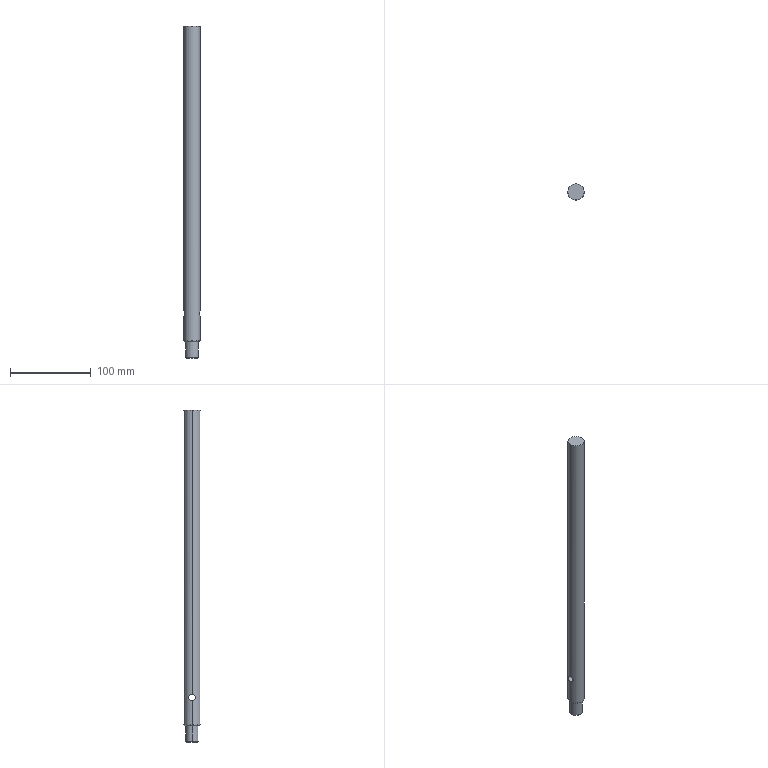Part | SolidWorks | features ICE 4, Chamfer 1, Revolution 1 | 1 solid | 13 faces | box 20 x 20 x 410 mm | volume 125504 mm3 | cylinder 6 | cone 4 | plane 3 | commonest cylinder face diameters 8 x2 16 x2 20 x2
STEP:
#1=CARTESIAN_POINT('',(-7.,0.,-190.));
#2=VERTEX_POINT('',#1);
#3=CARTESIAN_POINT('',(7.,0.,-190.));
#4=VERTEX_POINT('',#3);
#5=CARTESIAN_POINT('',(0.,0.,-190.));
#6=DIRECTION('',(0.,0.,-1.));
#7=DIRECTION('',(-1.,0.,0.));
#8=AXIS2_PLACEMENT_3D('',#5,#6,#7);
#9=CIRCLE('',#8,7.);
#10=EDGE_CURVE('',#2,#4,#9,.T.);
#11=ORIENTED_EDGE('',*,*,#10,.F.);
#12=CARTESIAN_POINT('',(-8.,0.,-189.));
#13=VERTEX_POINT('',#12);
#14=CARTESIAN_POINT('',(-7.,0.,-190.));
#15=DIRECTION('',(-0.7071,0.,0.7071));
#16=VECTOR('',#15,1000.);
#17=LINE('',#14,#16);
#18=EDGE_CURVE('',#2,#13,#17,.T.);
#19=ORIENTED_EDGE('',*,*,#18,.T.);
#20=CARTESIAN_POINT('',(8.,0.,-189.));
#21=VERTEX_POINT('',#20);
#22=CARTESIAN_POINT('',(0.,0.,-189.));
#23=DIRECTION('',(0.,0.,1.));
#24=DIRECTION('',(-1.,0.,0.));
#25=AXIS2_PLACEMENT_3D('',#22,#23,#24);
#26=CIRCLE('',#25,8.);
#27=EDGE_CURVE('',#21,#13,#26,.T.);
#28=ORIENTED_EDGE('',*,*,#27,.F.);
#29=CARTESIAN_POINT('',(7.,0.,-190.));
#30=DIRECTION('',(0.7071,0.,0.7071));
#31=VECTOR('',#30,1000.);
#32=LINE('',#29,#31);
#33=EDGE_CURVE('',#4,#21,#32,.T.);
#34=ORIENTED_EDGE('',*,*,#33,.F.);
#35=EDGE_LOOP('',(#11,#19,#28,#34));
#36=FACE_OUTER_BOUND('',#35,.T.);
#37=CARTESIAN_POINT('',(0.,0.,-190.));
#38=DIRECTION('',(0.,0.,1.));
#39=DIRECTION('',(1.,0.,0.));
#40=AXIS2_PLACEMENT_3D('',#37,#38,#39);
#41=CONICAL_SURFACE('',#40,7.,0.7854);
#42=ADVANCED_FACE('',(#36),#41,.T.);
#43=CARTESIAN_POINT('',(-9.,0.,-170.));
#44=VERTEX_POINT('',#43);
#45=CARTESIAN_POINT('',(9.,0.,-170.));
#46=VERTEX_POINT('',#45);
#47=CARTESIAN_POINT('',(0.,0.,-170.));
#48=DIRECTION('',(0.,0.,-1.));
#49=DIRECTION('',(-1.,0.,0.));
#50=AXIS2_PLACEMENT_3D('',#47,#48,#49);
#51=CIRCLE('',#50,9.);
#52=EDGE_CURVE('',#44,#46,#51,.T.);
#53=ORIENTED_EDGE('',*,*,#52,.F.);
#54=CARTESIAN_POINT('',(-10.,0.,-169.));
#55=VERTEX_POINT('',#54);
#56=CARTESIAN_POINT('',(-9.,0.,-170.));
#57=DIRECTION('',(-0.7071,0.,0.7071));
#58=VECTOR('',#57,1000.);
#59=LINE('',#56,#58);
#60=EDGE_CURVE('',#44,#55,#59,.T.);
#61=ORIENTED_EDGE('',*,*,#60,.T.);
#62=CARTESIAN_POINT('',(10.,0.,-169.));
#63=VERTEX_POINT('',#62);
#64=CARTESIAN_POINT('',(0.,0.,-169.));
#65=DIRECTION('',(0.,0.,1.));
#66=DIRECTION('',(-1.,0.,0.));
#67=AXIS2_PLACEMENT_3D('',#64,#65,#66);
#68=CIRCLE('',#67,10.);
#69=EDGE_CURVE('',#63,#55,#68,.T.);
#70=ORIENTED_EDGE('',*,*,#69,.F.);
#71=CARTESIAN_POINT('',(9.,0.,-170.));
#72=DIRECTION('',(0.7071,0.,0.7071));
#73=VECTOR('',#72,1000.);
#74=LINE('',#71,#73);
#75=EDGE_CURVE('',#46,#63,#74,.T.);
#76=ORIENTED_EDGE('',*,*,#75,.F.);
#77=EDGE_LOOP('',(#53,#61,#70,#76));
#78=FACE_OUTER_BOUND('',#77,.T.);
#79=CARTESIAN_POINT('',(0.,0.,-170.));
#80=DIRECTION('',(0.,0.,1.));
#81=DIRECTION('',(1.,0.,0.));
#82=AXIS2_PLACEMENT_3D('',#79,#80,#81);
#83=CONICAL_SURFACE('',#82,9.,0.7854);
#84=ADVANCED_FACE('',(#78),#83,.T.);
#85=ORIENTED_EDGE('',*,*,#27,.T.);
#86=CARTESIAN_POINT('',(-8.,0.,-170.));
#87=VERTEX_POINT('',#86);
#88=CARTESIAN_POINT('',(-8.,0.,-190.));
#89=DIRECTION('',(0.,0.,1.));
#90=VECTOR('',#89,1000.);
#91=LINE('',#88,#90);
#92=EDGE_CURVE('',#13,#87,#91,.T.);
#93=ORIENTED_EDGE('',*,*,#92,.T.);
#94=CARTESIAN_POINT('',(8.,0.,-170.));
#95=VERTEX_POINT('',#94);
#96=CARTESIAN_POINT('',(0.,0.,-170.));
#97=DIRECTION('',(0.,0.,-1.));
#98=DIRECTION('',(-1.,0.,0.));
#99=AXIS2_PLACEMENT_3D('',#96,#97,#98);
#100=CIRCLE('',#99,8.);
#101=EDGE_CURVE('',#87,#95,#100,.T.);
#102=ORIENTED_EDGE('',*,*,#101,.T.);
#103=CARTESIAN_POINT('',(8.,0.,-190.));
#104=DIRECTION('',(0.,0.,1.));
#105=VECTOR('',#104,1000.);
#106=LINE('',#103,#105);
#107=EDGE_CURVE('',#21,#95,#106,.T.);
#108=ORIENTED_EDGE('',*,*,#107,.F.);
#109=EDGE_LOOP('',(#85,#93,#102,#108));
#110=FACE_OUTER_BOUND('',#109,.T.);
#111=CARTESIAN_POINT('',(0.,0.,-190.));
#112=DIRECTION('',(0.,0.,1.));
#113=DIRECTION('',(1.,0.,0.));
#114=AXIS2_PLACEMENT_3D('',#111,#112,#113);
#115=CYLINDRICAL_SURFACE('',#114,8.);
#116=ADVANCED_FACE('',(#110),#115,.T.);
#117=CARTESIAN_POINT('',(10.,0.,-131.));
#118=VERTEX_POINT('',#117);
#119=CARTESIAN_POINT('',(10.,0.,-139.));
#120=VERTEX_POINT('',#119);
#121=CARTESIAN_POINT('',(10.,0.,-131.));
#122=CARTESIAN_POINT('',(10.,-0.2673,-131.));
#123=CARTESIAN_POINT('',(9.989,-0.5296,-131.027));
#124=CARTESIAN_POINT('',(9.949,-1.045,-131.13));
#125=CARTESIAN_POINT('',(9.918,-1.3,-131.208));
#126=CARTESIAN_POINT('',(9.843,-1.784,-131.41));
#127=CARTESIAN_POINT('',(9.798,-2.013,-131.533));
#128=CARTESIAN_POINT('',(9.699,-2.445,-131.824));
#129=CARTESIAN_POINT('',(9.645,-2.648,-131.991));
#130=CARTESIAN_POINT('',(9.537,-3.013,-132.356));
#131=CARTESIAN_POINT('',(9.483,-3.178,-132.556));
#132=CARTESIAN_POINT('',(9.38,-3.469,-132.991));
#133=CARTESIAN_POINT('',(9.333,-3.591,-133.22));
#134=CARTESIAN_POINT('',(9.254,-3.792,-133.7));
#135=CARTESIAN_POINT('',(9.221,-3.87,-133.954));
#136=CARTESIAN_POINT('',(9.177,-3.974,-134.472));
#137=CARTESIAN_POINT('',(9.165,-4.,-134.733));
#138=CARTESIAN_POINT('',(9.165,-4.,-135.262));
#139=CARTESIAN_POINT('',(9.177,-3.973,-135.53));
#140=CARTESIAN_POINT('',(9.221,-3.87,-136.045));
#141=CARTESIAN_POINT('',(9.253,-3.793,-136.297));
#142=CARTESIAN_POINT('',(9.334,-3.59,-136.784));
#143=CARTESIAN_POINT('',(9.381,-3.466,-137.013));
#144=CARTESIAN_POINT('',(9.483,-3.178,-137.443));
#145=CARTESIAN_POINT('',(9.538,-3.01,-137.646));
#146=CARTESIAN_POINT('',(9.646,-2.644,-138.012));
#147=CARTESIAN_POINT('',(9.699,-2.445,-138.176));
#148=CARTESIAN_POINT('',(9.798,-2.013,-138.466));
#149=CARTESIAN_POINT('',(9.843,-1.78,-138.592));
#150=CARTESIAN_POINT('',(9.918,-1.299,-138.792));
#151=CARTESIAN_POINT('',(9.948,-1.049,-138.869));
#152=CARTESIAN_POINT('',(9.99,-0.5273,-138.974));
#153=CARTESIAN_POINT('',(10.,-0.2633,-139.));
#154=CARTESIAN_POINT('',(10.,0.,-139.));
#155=B_SPLINE_CURVE_WITH_KNOTS('',3,(#121,#122,#123,#124,#125,#126,#127,#128,#129,#130,#131,#132,#133,#134,#135,#136,#137,#138,#139,#140,#141,#142,#143,#144,#145,#146,#147,#148,#149,#150,#151,#152,#153,#154),.UNSPECIFIED.,.F.,.F.,(4,2,2,2,2,2,2,2,2,2,2,2,2,2,2,2,4),(0.,0.00079,0.00158,0.00237,0.00316,0.00395,0.00474,0.00553,0.00632,0.00711,0.0079,0.00869,0.00948,0.01027,0.01106,0.01185,0.01264),.UNSPECIFIED.);
#156=EDGE_CURVE('',#118,#120,#155,.T.);
#157=ORIENTED_EDGE('',*,*,#156,.T.);
#158=CARTESIAN_POINT('',(-10.,0.,-139.));
#159=VERTEX_POINT('',#158);
#160=CARTESIAN_POINT('',(10.,0.,-139.));
#161=DIRECTION('',(-1.,0.,0.));
#162=VECTOR('',#161,1000.);
#163=LINE('',#160,#162);
#164=EDGE_CURVE('',#120,#159,#163,.T.);
#165=ORIENTED_EDGE('',*,*,#164,.T.);
#166=CARTESIAN_POINT('',(-10.,0.,-131.));
#167=VERTEX_POINT('',#166);
#168=CARTESIAN_POINT('',(-10.,0.,-139.));
#169=CARTESIAN_POINT('',(-10.,-0.2631,-139.));
#170=CARTESIAN_POINT('',(-9.989,-0.5298,-138.974));
#171=CARTESIAN_POINT('',(-9.948,-1.048,-138.869));
#172=CARTESIAN_POINT('',(-9.918,-1.299,-138.792));
#173=CARTESIAN_POINT('',(-9.843,-1.782,-138.591));
#174=CARTESIAN_POINT('',(-9.797,-2.015,-138.465));
#175=CARTESIAN_POINT('',(-9.699,-2.446,-138.176));
#176=CARTESIAN_POINT('',(-9.645,-2.646,-138.011));
#177=CARTESIAN_POINT('',(-9.537,-3.015,-137.642));
#178=CARTESIAN_POINT('',(-9.483,-3.179,-137.442));
#179=CARTESIAN_POINT('',(-9.381,-3.466,-137.013));
#180=CARTESIAN_POINT('',(-9.333,-3.592,-136.78));
#181=CARTESIAN_POINT('',(-9.253,-3.793,-136.297));
#182=CARTESIAN_POINT('',(-9.221,-3.869,-136.048));
#183=CARTESIAN_POINT('',(-9.177,-3.973,-135.532));
#184=CARTESIAN_POINT('',(-9.165,-4.,-135.264));
#185=CARTESIAN_POINT('',(-9.165,-4.,-134.737));
#186=CARTESIAN_POINT('',(-9.177,-3.974,-134.475));
#187=CARTESIAN_POINT('',(-9.221,-3.87,-133.954));
#188=CARTESIAN_POINT('',(-9.254,-3.792,-133.702));
#189=CARTESIAN_POINT('',(-9.333,-3.592,-133.22));
#190=CARTESIAN_POINT('',(-9.381,-3.467,-132.987));
#191=CARTESIAN_POINT('',(-9.483,-3.177,-132.556));
#192=CARTESIAN_POINT('',(-9.537,-3.013,-132.356));
#193=CARTESIAN_POINT('',(-9.645,-2.646,-131.989));
#194=CARTESIAN_POINT('',(-9.699,-2.443,-131.822));
#195=CARTESIAN_POINT('',(-9.798,-2.014,-131.534));
#196=CARTESIAN_POINT('',(-9.842,-1.785,-131.411));
#197=CARTESIAN_POINT('',(-9.918,-1.298,-131.207));
#198=CARTESIAN_POINT('',(-9.948,-1.046,-131.13));
#199=CARTESIAN_POINT('',(-9.989,-0.5323,-131.027));
#200=CARTESIAN_POINT('',(-10.,-0.2671,-131.));
#201=CARTESIAN_POINT('',(-10.,0.,-131.));
#202=B_SPLINE_CURVE_WITH_KNOTS('',3,(#168,#169,#170,#171,#172,#173,#174,#175,#176,#177,#178,#179,#180,#181,#182,#183,#184,#185,#186,#187,#188,#189,#190,#191,#192,#193,#194,#195,#196,#197,#198,#199,#200,#201),.UNSPECIFIED.,.F.,.F.,(4,2,2,2,2,2,2,2,2,2,2,2,2,2,2,2,4),(0.01264,0.01343,0.01422,0.01501,0.0158,0.01659,0.01738,0.01817,0.01896,0.01974,0.02053,0.02132,0.02211,0.0229,0.02369,0.02448,0.02527),.UNSPECIFIED.);
#203=EDGE_CURVE('',#159,#167,#202,.T.);
#204=ORIENTED_EDGE('',*,*,#203,.T.);
#205=CARTESIAN_POINT('',(10.,0.,-131.));
#206=DIRECTION('',(-1.,0.,0.));
#207=VECTOR('',#206,1000.);
#208=LINE('',#205,#207);
#209=EDGE_CURVE('',#118,#167,#208,.T.);
#210=ORIENTED_EDGE('',*,*,#209,.F.);
#211=EDGE_LOOP('',(#157,#165,#204,#210));
#212=FACE_OUTER_BOUND('',#211,.T.);
#213=CARTESIAN_POINT('',(10.,0.,-135.));
#214=DIRECTION('',(-1.,0.,0.));
#215=DIRECTION('',(0.,0.,1.));
#216=AXIS2_PLACEMENT_3D('',#213,#214,#215);
#217=CYLINDRICAL_SURFACE('',#216,4.);
#218=ADVANCED_FACE('',(#212),#217,.F.);
#219=ORIENTED_EDGE('',*,*,#69,.T.);
#220=CARTESIAN_POINT('',(-10.,0.,0.));
#221=DIRECTION('',(0.,0.,1.));
#222=VECTOR('',#221,1000.);
#223=LINE('',#220,#222);
#224=EDGE_CURVE('',#55,#159,#223,.T.);
#225=ORIENTED_EDGE('',*,*,#224,.T.);
#226=CARTESIAN_POINT('',(-10.,0.,-131.));
#227=CARTESIAN_POINT('',(-10.,0.2673,-131.));
#228=CARTESIAN_POINT('',(-9.989,0.5296,-131.027));
#229=CARTESIAN_POINT('',(-9.949,1.045,-131.13));
#230=CARTESIAN_POINT('',(-9.918,1.3,-131.208));
#231=CARTESIAN_POINT('',(-9.843,1.784,-131.41));
#232=CARTESIAN_POINT('',(-9.798,2.013,-131.533));
#233=CARTESIAN_POINT('',(-9.699,2.445,-131.824));
#234=CARTESIAN_POINT('',(-9.645,2.648,-131.991));
#235=CARTESIAN_POINT('',(-9.537,3.013,-132.356));
#236=CARTESIAN_POINT('',(-9.483,3.178,-132.556));
#237=CARTESIAN_POINT('',(-9.38,3.469,-132.991));
#238=CARTESIAN_POINT('',(-9.333,3.591,-133.22));
#239=CARTESIAN_POINT('',(-9.254,3.792,-133.7));
#240=CARTESIAN_POINT('',(-9.221,3.87,-133.954));
#241=CARTESIAN_POINT('',(-9.177,3.974,-134.472));
#242=CARTESIAN_POINT('',(-9.165,4.,-134.733));
#243=CARTESIAN_POINT('',(-9.165,4.,-135.262));
#244=CARTESIAN_POINT('',(-9.177,3.973,-135.53));
#245=CARTESIAN_POINT('',(-9.221,3.87,-136.045));
#246=CARTESIAN_POINT('',(-9.253,3.793,-136.297));
#247=CARTESIAN_POINT('',(-9.334,3.59,-136.784));
#248=CARTESIAN_POINT('',(-9.381,3.466,-137.013));
#249=CARTESIAN_POINT('',(-9.483,3.178,-137.443));
#250=CARTESIAN_POINT('',(-9.538,3.01,-137.646));
#251=CARTESIAN_POINT('',(-9.646,2.644,-138.012));
#252=CARTESIAN_POINT('',(-9.699,2.445,-138.176));
#253=CARTESIAN_POINT('',(-9.798,2.013,-138.466));
#254=CARTESIAN_POINT('',(-9.843,1.78,-138.592));
#255=CARTESIAN_POINT('',(-9.918,1.299,-138.792));
#256=CARTESIAN_POINT('',(-9.948,1.049,-138.869));
#257=CARTESIAN_POINT('',(-9.99,0.5273,-138.974));
#258=CARTESIAN_POINT('',(-10.,0.2633,-139.));
#259=CARTESIAN_POINT('',(-10.,0.,-139.));
#260=B_SPLINE_CURVE_WITH_KNOTS('',3,(#226,#227,#228,#229,#230,#231,#232,#233,#234,#235,#236,#237,#238,#239,#240,#241,#242,#243,#244,#245,#246,#247,#248,#249,#250,#251,#252,#253,#254,#255,#256,#257,#258,#259),.UNSPECIFIED.,.F.,.F.,(4,2,2,2,2,2,2,2,2,2,2,2,2,2,2,2,4),(0.,0.00079,0.00158,0.00237,0.00316,0.00395,0.00474,0.00553,0.00632,0.00711,0.0079,0.00869,0.00948,0.01027,0.01106,0.01185,0.01264),.UNSPECIFIED.);
#261=EDGE_CURVE('',#167,#159,#260,.T.);
#262=ORIENTED_EDGE('',*,*,#261,.F.);
#263=CARTESIAN_POINT('',(-10.,0.,220.));
#264=VERTEX_POINT('',#263);
#265=CARTESIAN_POINT('',(-10.,0.,0.));
#266=DIRECTION('',(0.,0.,1.));
#267=VECTOR('',#266,1000.);
#268=LINE('',#265,#267);
#269=EDGE_CURVE('',#167,#264,#268,.T.);
#270=ORIENTED_EDGE('',*,*,#269,.T.);
#271=CARTESIAN_POINT('',(10.,0.,220.));
#272=VERTEX_POINT('',#271);
#273=CARTESIAN_POINT('',(0.,0.,220.));
#274=DIRECTION('',(0.,0.,1.));
#275=DIRECTION('',(1.,0.,0.));
#276=AXIS2_PLACEMENT_3D('',#273,#274,#275);
#277=CIRCLE('',#276,10.);
#278=EDGE_CURVE('',#272,#264,#277,.T.);
#279=ORIENTED_EDGE('',*,*,#278,.F.);
#280=CARTESIAN_POINT('',(10.,0.,0.));
#281=DIRECTION('',(0.,0.,1.));
#282=VECTOR('',#281,1000.);
#283=LINE('',#280,#282);
#284=EDGE_CURVE('',#118,#272,#283,.T.);
#285=ORIENTED_EDGE('',*,*,#284,.F.);
#286=CARTESIAN_POINT('',(10.,0.,-139.));
#287=CARTESIAN_POINT('',(10.,0.2631,-139.));
#288=CARTESIAN_POINT('',(9.989,0.5298,-138.974));
#289=CARTESIAN_POINT('',(9.948,1.048,-138.869));
#290=CARTESIAN_POINT('',(9.918,1.299,-138.792));
#291=CARTESIAN_POINT('',(9.843,1.782,-138.591));
#292=CARTESIAN_POINT('',(9.797,2.015,-138.465));
#293=CARTESIAN_POINT('',(9.699,2.446,-138.176));
#294=CARTESIAN_POINT('',(9.645,2.646,-138.011));
#295=CARTESIAN_POINT('',(9.537,3.015,-137.642));
#296=CARTESIAN_POINT('',(9.483,3.179,-137.442));
#297=CARTESIAN_POINT('',(9.381,3.466,-137.013));
#298=CARTESIAN_POINT('',(9.333,3.592,-136.78));
#299=CARTESIAN_POINT('',(9.253,3.793,-136.297));
#300=CARTESIAN_POINT('',(9.221,3.869,-136.048));
#301=CARTESIAN_POINT('',(9.177,3.973,-135.532));
#302=CARTESIAN_POINT('',(9.165,4.,-135.264));
#303=CARTESIAN_POINT('',(9.165,4.,-134.737));
#304=CARTESIAN_POINT('',(9.177,3.974,-134.475));
#305=CARTESIAN_POINT('',(9.221,3.87,-133.954));
#306=CARTESIAN_POINT('',(9.254,3.792,-133.702));
#307=CARTESIAN_POINT('',(9.333,3.592,-133.22));
#308=CARTESIAN_POINT('',(9.381,3.467,-132.987));
#309=CARTESIAN_POINT('',(9.483,3.177,-132.556));
#310=CARTESIAN_POINT('',(9.537,3.013,-132.356));
#311=CARTESIAN_POINT('',(9.645,2.646,-131.989));
#312=CARTESIAN_POINT('',(9.699,2.443,-131.822));
#313=CARTESIAN_POINT('',(9.798,2.014,-131.534));
#314=CARTESIAN_POINT('',(9.842,1.785,-131.411));
#315=CARTESIAN_POINT('',(9.918,1.298,-131.207));
#316=CARTESIAN_POINT('',(9.948,1.046,-131.13));
#317=CARTESIAN_POINT('',(9.989,0.5323,-131.027));
#318=CARTESIAN_POINT('',(10.,0.2671,-131.));
#319=CARTESIAN_POINT('',(10.,0.,-131.));
#320=B_SPLINE_CURVE_WITH_KNOTS('',3,(#286,#287,#288,#289,#290,#291,#292,#293,#294,#295,#296,#297,#298,#299,#300,#301,#302,#303,#304,#305,#306,#307,#308,#309,#310,#311,#312,#313,#314,#315,#316,#317,#318,#319),.UNSPECIFIED.,.F.,.F.,(4,2,2,2,2,2,2,2,2,2,2,2,2,2,2,2,4),(0.01264,0.01343,0.01422,0.01501,0.0158,0.01659,0.01738,0.01817,0.01896,0.01974,0.02053,0.02132,0.02211,0.0229,0.02369,0.02448,0.02527),.UNSPECIFIED.);
#321=EDGE_CURVE('',#120,#118,#320,.T.);
#322=ORIENTED_EDGE('',*,*,#321,.F.);
#323=CARTESIAN_POINT('',(10.,0.,0.));
#324=DIRECTION('',(0.,0.,1.));
#325=VECTOR('',#324,1000.);
#326=LINE('',#323,#325);
#327=EDGE_CURVE('',#63,#120,#326,.T.);
#328=ORIENTED_EDGE('',*,*,#327,.F.);
#329=EDGE_LOOP('',(#219,#225,#262,#270,#279,#285,#322,#328));
#330=FACE_OUTER_BOUND('',#329,.T.);
#331=CARTESIAN_POINT('',(0.,0.,0.));
#332=DIRECTION('',(0.,0.,1.));
#333=DIRECTION('',(1.,0.,0.));
#334=AXIS2_PLACEMENT_3D('',#331,#332,#333);
#335=CYLINDRICAL_SURFACE('',#334,10.);
#336=ADVANCED_FACE('',(#330),#335,.T.);
#337=ORIENTED_EDGE('',*,*,#224,.F.);
#338=CARTESIAN_POINT('',(0.,0.,-169.));
#339=DIRECTION('',(0.,0.,1.));
#340=DIRECTION('',(-1.,0.,0.));
#341=AXIS2_PLACEMENT_3D('',#338,#339,#340);
#342=CIRCLE('',#341,10.);
#343=EDGE_CURVE('',#55,#63,#342,.T.);
#344=ORIENTED_EDGE('',*,*,#343,.T.);
#345=ORIENTED_EDGE('',*,*,#327,.T.);
#346=ORIENTED_EDGE('',*,*,#156,.F.);
#347=ORIENTED_EDGE('',*,*,#284,.T.);
#348=CARTESIAN_POINT('',(0.,0.,220.));
#349=DIRECTION('',(0.,0.,1.));
#350=DIRECTION('',(1.,0.,0.));
#351=AXIS2_PLACEMENT_3D('',#348,#349,#350);
#352=CIRCLE('',#351,10.);
#353=EDGE_CURVE('',#264,#272,#352,.T.);
#354=ORIENTED_EDGE('',*,*,#353,.F.);
#355=ORIENTED_EDGE('',*,*,#269,.F.);
#356=ORIENTED_EDGE('',*,*,#203,.F.);
#357=EDGE_LOOP('',(#337,#344,#345,#346,#347,#354,#355,#356));
#358=FACE_OUTER_BOUND('',#357,.T.);
#359=CARTESIAN_POINT('',(0.,0.,0.));
#360=DIRECTION('',(0.,0.,1.));
#361=DIRECTION('',(1.,0.,0.));
#362=AXIS2_PLACEMENT_3D('',#359,#360,#361);
#363=CYLINDRICAL_SURFACE('',#362,10.);
#364=ADVANCED_FACE('',(#358),#363,.T.);
#365=ORIENTED_EDGE('',*,*,#164,.F.);
#366=ORIENTED_EDGE('',*,*,#321,.T.);
#367=ORIENTED_EDGE('',*,*,#209,.T.);
#368=ORIENTED_EDGE('',*,*,#261,.T.);
#369=EDGE_LOOP('',(#365,#366,#367,#368));
#370=FACE_OUTER_BOUND('',#369,.T.);
#371=CARTESIAN_POINT('',(10.,0.,-135.));
#372=DIRECTION('',(-1.,0.,0.));
#373=DIRECTION('',(0.,0.,1.));
#374=AXIS2_PLACEMENT_3D('',#371,#372,#373);
#375=CYLINDRICAL_SURFACE('',#374,4.);
#376=ADVANCED_FACE('',(#370),#375,.F.);
#377=CARTESIAN_POINT('',(0.,0.,-170.));
#378=DIRECTION('',(0.,0.,-1.));
#379=DIRECTION('',(-1.,0.,0.));
#380=AXIS2_PLACEMENT_3D('',#377,#378,#379);
#381=CIRCLE('',#380,9.);
#382=EDGE_CURVE('',#46,#44,#381,.T.);
#383=ORIENTED_EDGE('',*,*,#382,.T.);
#384=ORIENTED_EDGE('',*,*,#52,.T.);
#385=EDGE_LOOP('',(#383,#384));
#386=FACE_OUTER_BOUND('',#385,.T.);
#387=CARTESIAN_POINT('',(0.,0.,-170.));
#388=DIRECTION('',(0.,0.,-1.));
#389=DIRECTION('',(-1.,0.,0.));
#390=AXIS2_PLACEMENT_3D('',#387,#388,#389);
#391=CIRCLE('',#390,8.);
#392=EDGE_CURVE('',#95,#87,#391,.T.);
#393=ORIENTED_EDGE('',*,*,#392,.F.);
#394=ORIENTED_EDGE('',*,*,#101,.F.);
#395=EDGE_LOOP('',(#393,#394));
#396=FACE_BOUND('',#395,.T.);
#397=CARTESIAN_POINT('',(0.,0.,-170.));
#398=DIRECTION('',(0.,0.,-1.));
#399=DIRECTION('',(-1.,0.,0.));
#400=AXIS2_PLACEMENT_3D('',#397,#398,#399);
#401=PLANE('',#400);
#402=ADVANCED_FACE('',(#386,#396),#401,.T.);
#403=ORIENTED_EDGE('',*,*,#92,.F.);
#404=CARTESIAN_POINT('',(0.,0.,-189.));
#405=DIRECTION('',(0.,0.,1.));
#406=DIRECTION('',(-1.,0.,0.));
#407=AXIS2_PLACEMENT_3D('',#404,#405,#406);
#408=CIRCLE('',#407,8.);
#409=EDGE_CURVE('',#13,#21,#408,.T.);
#410=ORIENTED_EDGE('',*,*,#409,.T.);
#411=ORIENTED_EDGE('',*,*,#107,.T.);
#412=ORIENTED_EDGE('',*,*,#392,.T.);
#413=EDGE_LOOP('',(#403,#410,#411,#412));
#414=FACE_OUTER_BOUND('',#413,.T.);
#415=CARTESIAN_POINT('',(0.,0.,-190.));
#416=DIRECTION('',(0.,0.,1.));
#417=DIRECTION('',(1.,0.,0.));
#418=AXIS2_PLACEMENT_3D('',#415,#416,#417);
#419=CYLINDRICAL_SURFACE('',#418,8.);
#420=ADVANCED_FACE('',(#414),#419,.T.);
#421=CARTESIAN_POINT('',(0.,0.,-190.));
#422=DIRECTION('',(0.,0.,-1.));
#423=DIRECTION('',(-1.,0.,0.));
#424=AXIS2_PLACEMENT_3D('',#421,#422,#423);
#425=CIRCLE('',#424,7.);
#426=EDGE_CURVE('',#4,#2,#425,.T.);
#427=ORIENTED_EDGE('',*,*,#426,.T.);
#428=ORIENTED_EDGE('',*,*,#10,.T.);
#429=EDGE_LOOP('',(#427,#428));
#430=FACE_OUTER_BOUND('',#429,.T.);
#431=CARTESIAN_POINT('',(0.,0.,-190.));
#432=DIRECTION('',(0.,0.,-1.));
#433=DIRECTION('',(-1.,0.,0.));
#434=AXIS2_PLACEMENT_3D('',#431,#432,#433);
#435=PLANE('',#434);
#436=ADVANCED_FACE('',(#430),#435,.T.);
#437=ORIENTED_EDGE('',*,*,#60,.F.);
#438=ORIENTED_EDGE('',*,*,#382,.F.);
#439=ORIENTED_EDGE('',*,*,#75,.T.);
#440=ORIENTED_EDGE('',*,*,#343,.F.);
#441=EDGE_LOOP('',(#437,#438,#439,#440));
#442=FACE_OUTER_BOUND('',#441,.T.);
#443=CARTESIAN_POINT('',(0.,0.,-170.));
#444=DIRECTION('',(0.,0.,1.));
#445=DIRECTION('',(1.,0.,0.));
#446=AXIS2_PLACEMENT_3D('',#443,#444,#445);
#447=CONICAL_SURFACE('',#446,9.,0.7854);
#448=ADVANCED_FACE('',(#442),#447,.T.);
#449=ORIENTED_EDGE('',*,*,#18,.F.);
#450=ORIENTED_EDGE('',*,*,#426,.F.);
#451=ORIENTED_EDGE('',*,*,#33,.T.);
#452=ORIENTED_EDGE('',*,*,#409,.F.);
#453=EDGE_LOOP('',(#449,#450,#451,#452));
#454=FACE_OUTER_BOUND('',#453,.T.);
#455=CARTESIAN_POINT('',(0.,0.,-190.));
#456=DIRECTION('',(0.,0.,1.));
#457=DIRECTION('',(1.,0.,0.));
#458=AXIS2_PLACEMENT_3D('',#455,#456,#457);
#459=CONICAL_SURFACE('',#458,7.,0.7854);
#460=ADVANCED_FACE('',(#454),#459,.T.);
#461=ORIENTED_EDGE('',*,*,#278,.T.);
#462=ORIENTED_EDGE('',*,*,#353,.T.);
#463=EDGE_LOOP('',(#461,#462));
#464=FACE_OUTER_BOUND('',#463,.T.);
#465=CARTESIAN_POINT('',(0.,0.,220.));
#466=DIRECTION('',(0.,0.,1.));
#467=DIRECTION('',(1.,0.,0.));
#468=AXIS2_PLACEMENT_3D('',#465,#466,#467);
#469=PLANE('',#468);
#470=ADVANCED_FACE('',(#464),#469,.T.);
#471=CLOSED_SHELL('',(#42,#84,#116,#218,#336,#364,#376,#402,#420,#436,#448,#460,#470));
#472=MANIFOLD_SOLID_BREP('',#471);
#473=CARTESIAN_POINT('',(0.,0.,0.));
#474=DIRECTION('',(0.,0.,1.));
#475=DIRECTION('',(1.,0.,0.));
#476=AXIS2_PLACEMENT_3D('',#473,#474,#475);
#477=(LENGTH_UNIT()NAMED_UNIT(*)SI_UNIT(.MILLI.,.METRE.));
#478=UNCERTAINTY_MEASURE_WITH_UNIT(LENGTH_MEASURE(0.00001),#477,'','');
#479=(NAMED_UNIT(*)PLANE_ANGLE_UNIT()SI_UNIT($,.RADIAN.));
#480=(NAMED_UNIT(*)SI_UNIT($,.STERADIAN.)SOLID_ANGLE_UNIT());
#481=(GEOMETRIC_REPRESENTATION_CONTEXT(3)GLOBAL_UNCERTAINTY_ASSIGNED_CONTEXT((#478))GLOBAL_UNIT_ASSIGNED_CONTEXT((#477,#479,#480))REPRESENTATION_CONTEXT('',''));
#482=ADVANCED_BREP_SHAPE_REPRESENTATION('',(#472,#476),#481);